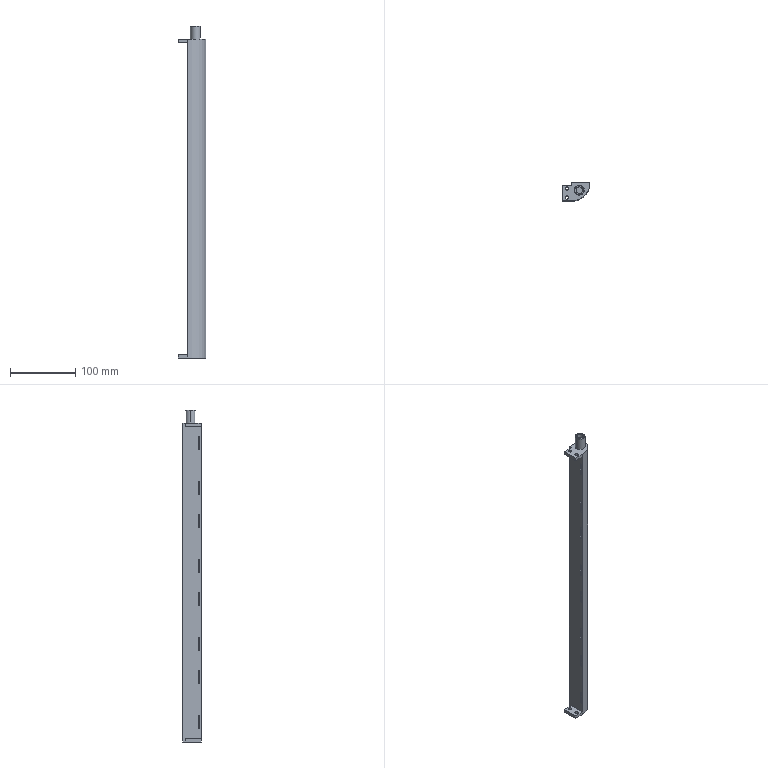Part | SolidWorks | features BaseBody 1 | 1 solid | 65 faces | box 43 x 28 x 510 mm | volume 99818 mm3 | plane 49 | cylinder 14 | cone 2 | commonest cylinder face diameters 5 x8 10 x2 15 x2 52 x1 56 x1